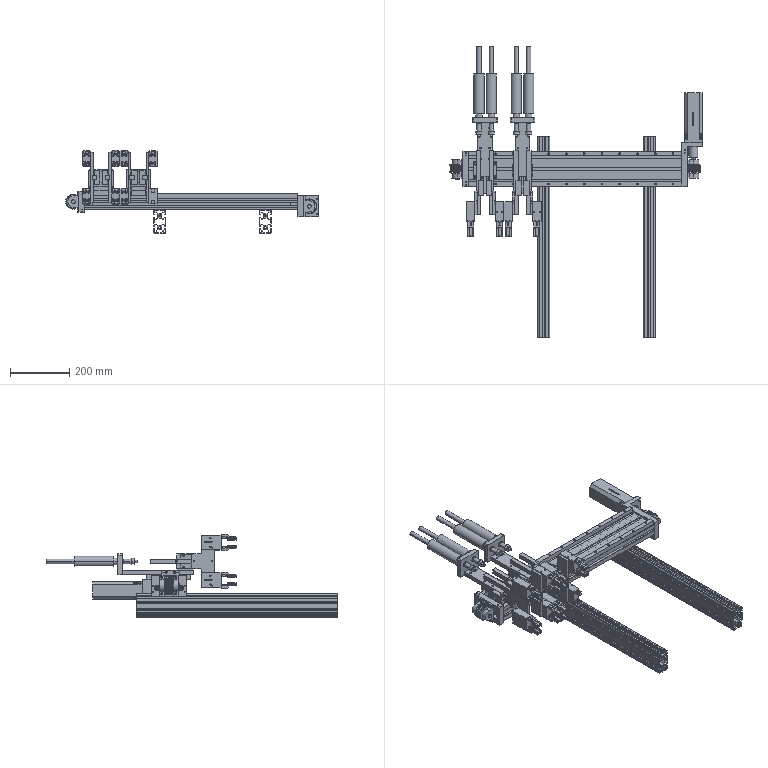Part | 93 solids | 6343 faces | volume 7238932 mm3 | plane 3659 | cylinder 1409 | spline 1097 | cone 178 | commonest cylinder face diameters 3.3 x208 35 x192 5 x172 0.96 x140 1.14 x80 4.2 x72